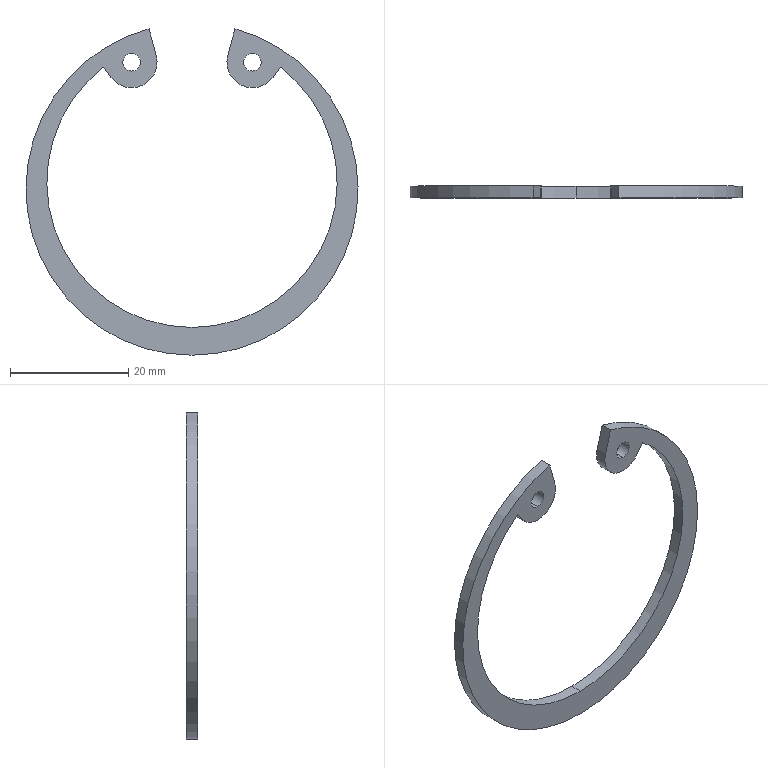Part | SolidWorks | features Extrusion 1 | 1 solid | 18 faces | box 56.2 x 2 x 55.243 mm | volume 1250 mm3 | cylinder 12 | plane 6 | commonest cylinder face diameters 3 x4 8.62 x4 49.15 x2 56.2 x2
STEP:
#1=CARTESIAN_POINT('',(10.219,2.,19.984));
#2=VERTEX_POINT('',#1);
#3=CARTESIAN_POINT('',(10.219,2.,22.984));
#4=VERTEX_POINT('',#3);
#5=CARTESIAN_POINT('',(10.219,2.,21.484));
#6=DIRECTION('',(0.,1.,0.));
#7=DIRECTION('',(0.,0.,-1.));
#8=AXIS2_PLACEMENT_3D('',#5,#6,#7);
#9=CIRCLE('',#8,1.5);
#10=EDGE_CURVE('',#2,#4,#9,.T.);
#11=ORIENTED_EDGE('',*,*,#10,.T.);
#12=CARTESIAN_POINT('',(10.219,0.,22.984));
#13=VERTEX_POINT('',#12);
#14=CARTESIAN_POINT('',(10.219,2.,22.984));
#15=DIRECTION('',(0.,-1.,0.));
#16=VECTOR('',#15,1000.);
#17=LINE('',#14,#16);
#18=EDGE_CURVE('',#4,#13,#17,.T.);
#19=ORIENTED_EDGE('',*,*,#18,.T.);
#20=CARTESIAN_POINT('',(10.219,0.,19.984));
#21=VERTEX_POINT('',#20);
#22=CARTESIAN_POINT('',(10.219,0.,21.484));
#23=DIRECTION('',(0.,1.,0.));
#24=DIRECTION('',(0.,0.,-1.));
#25=AXIS2_PLACEMENT_3D('',#22,#23,#24);
#26=CIRCLE('',#25,1.5);
#27=EDGE_CURVE('',#21,#13,#26,.T.);
#28=ORIENTED_EDGE('',*,*,#27,.F.);
#29=CARTESIAN_POINT('',(10.219,2.,19.984));
#30=DIRECTION('',(0.,-1.,0.));
#31=VECTOR('',#30,1000.);
#32=LINE('',#29,#31);
#33=EDGE_CURVE('',#2,#21,#32,.T.);
#34=ORIENTED_EDGE('',*,*,#33,.F.);
#35=EDGE_LOOP('',(#11,#19,#28,#34));
#36=FACE_OUTER_BOUND('',#35,.T.);
#37=CARTESIAN_POINT('',(10.219,2.,21.484));
#38=DIRECTION('',(0.,-1.,0.));
#39=DIRECTION('',(0.,0.,-1.));
#40=AXIS2_PLACEMENT_3D('',#37,#38,#39);
#41=CYLINDRICAL_SURFACE('',#40,1.5);
#42=ADVANCED_FACE('',(#36),#41,.F.);
#43=CARTESIAN_POINT('',(-10.219,2.,19.984));
#44=VERTEX_POINT('',#43);
#45=CARTESIAN_POINT('',(-10.219,2.,22.984));
#46=VERTEX_POINT('',#45);
#47=CARTESIAN_POINT('',(-10.219,2.,21.484));
#48=DIRECTION('',(0.,1.,0.));
#49=DIRECTION('',(0.,0.,1.));
#50=AXIS2_PLACEMENT_3D('',#47,#48,#49);
#51=CIRCLE('',#50,1.5);
#52=EDGE_CURVE('',#44,#46,#51,.T.);
#53=ORIENTED_EDGE('',*,*,#52,.T.);
#54=CARTESIAN_POINT('',(-10.219,0.,22.984));
#55=VERTEX_POINT('',#54);
#56=CARTESIAN_POINT('',(-10.219,2.,22.984));
#57=DIRECTION('',(0.,-1.,0.));
#58=VECTOR('',#57,1000.);
#59=LINE('',#56,#58);
#60=EDGE_CURVE('',#46,#55,#59,.T.);
#61=ORIENTED_EDGE('',*,*,#60,.T.);
#62=CARTESIAN_POINT('',(-10.219,0.,19.984));
#63=VERTEX_POINT('',#62);
#64=CARTESIAN_POINT('',(-10.219,0.,21.484));
#65=DIRECTION('',(0.,1.,0.));
#66=DIRECTION('',(0.,0.,1.));
#67=AXIS2_PLACEMENT_3D('',#64,#65,#66);
#68=CIRCLE('',#67,1.5);
#69=EDGE_CURVE('',#63,#55,#68,.T.);
#70=ORIENTED_EDGE('',*,*,#69,.F.);
#71=CARTESIAN_POINT('',(-10.219,2.,19.984));
#72=DIRECTION('',(0.,-1.,0.));
#73=VECTOR('',#72,1000.);
#74=LINE('',#71,#73);
#75=EDGE_CURVE('',#44,#63,#74,.T.);
#76=ORIENTED_EDGE('',*,*,#75,.F.);
#77=EDGE_LOOP('',(#53,#61,#70,#76));
#78=FACE_OUTER_BOUND('',#77,.T.);
#79=CARTESIAN_POINT('',(-10.219,2.,21.484));
#80=DIRECTION('',(0.,-1.,0.));
#81=DIRECTION('',(0.,0.,-1.));
#82=AXIS2_PLACEMENT_3D('',#79,#80,#81);
#83=CYLINDRICAL_SURFACE('',#82,1.5);
#84=ADVANCED_FACE('',(#78),#83,.F.);
#85=CARTESIAN_POINT('',(0.,2.,-28.1));
#86=VERTEX_POINT('',#85);
#87=CARTESIAN_POINT('',(-7.273,2.,27.143));
#88=VERTEX_POINT('',#87);
#89=CARTESIAN_POINT('',(0.,2.,0.));
#90=DIRECTION('',(0.,1.,0.));
#91=DIRECTION('',(0.,0.,1.));
#92=AXIS2_PLACEMENT_3D('',#89,#90,#91);
#93=CIRCLE('',#92,28.1);
#94=EDGE_CURVE('',#86,#88,#93,.T.);
#95=ORIENTED_EDGE('',*,*,#94,.F.);
#96=CARTESIAN_POINT('',(0.,0.,-28.1));
#97=VERTEX_POINT('',#96);
#98=CARTESIAN_POINT('',(0.,2.,-28.1));
#99=DIRECTION('',(0.,-1.,0.));
#100=VECTOR('',#99,1000.);
#101=LINE('',#98,#100);
#102=EDGE_CURVE('',#86,#97,#101,.T.);
#103=ORIENTED_EDGE('',*,*,#102,.T.);
#104=CARTESIAN_POINT('',(-7.273,0.,27.143));
#105=VERTEX_POINT('',#104);
#106=CARTESIAN_POINT('',(0.,0.,0.));
#107=DIRECTION('',(0.,1.,0.));
#108=DIRECTION('',(0.,0.,1.));
#109=AXIS2_PLACEMENT_3D('',#106,#107,#108);
#110=CIRCLE('',#109,28.1);
#111=EDGE_CURVE('',#97,#105,#110,.T.);
#112=ORIENTED_EDGE('',*,*,#111,.T.);
#113=CARTESIAN_POINT('',(-7.273,2.,27.143));
#114=DIRECTION('',(0.,-1.,0.));
#115=VECTOR('',#114,1000.);
#116=LINE('',#113,#115);
#117=EDGE_CURVE('',#88,#105,#116,.T.);
#118=ORIENTED_EDGE('',*,*,#117,.F.);
#119=EDGE_LOOP('',(#95,#103,#112,#118));
#120=FACE_OUTER_BOUND('',#119,.T.);
#121=CARTESIAN_POINT('',(0.,2.,0.));
#122=DIRECTION('',(0.,-1.,0.));
#123=DIRECTION('',(0.,0.,-1.));
#124=AXIS2_PLACEMENT_3D('',#121,#122,#123);
#125=CYLINDRICAL_SURFACE('',#124,28.1);
#126=ADVANCED_FACE('',(#120),#125,.T.);
#127=CARTESIAN_POINT('',(10.219,2.,17.174));
#128=VERTEX_POINT('',#127);
#129=CARTESIAN_POINT('',(6.055,2.,22.599));
#130=VERTEX_POINT('',#129);
#131=CARTESIAN_POINT('',(10.219,2.,21.484));
#132=DIRECTION('',(0.,1.,0.));
#133=DIRECTION('',(0.,0.,-1.));
#134=AXIS2_PLACEMENT_3D('',#131,#132,#133);
#135=CIRCLE('',#134,4.31);
#136=EDGE_CURVE('',#128,#130,#135,.T.);
#137=ORIENTED_EDGE('',*,*,#136,.F.);
#138=CARTESIAN_POINT('',(10.219,0.,17.174));
#139=VERTEX_POINT('',#138);
#140=CARTESIAN_POINT('',(10.219,2.,17.174));
#141=DIRECTION('',(0.,-1.,0.));
#142=VECTOR('',#141,1000.);
#143=LINE('',#140,#142);
#144=EDGE_CURVE('',#128,#139,#143,.T.);
#145=ORIENTED_EDGE('',*,*,#144,.T.);
#146=CARTESIAN_POINT('',(6.055,0.,22.599));
#147=VERTEX_POINT('',#146);
#148=CARTESIAN_POINT('',(10.219,0.,21.484));
#149=DIRECTION('',(0.,1.,0.));
#150=DIRECTION('',(0.,0.,-1.));
#151=AXIS2_PLACEMENT_3D('',#148,#149,#150);
#152=CIRCLE('',#151,4.31);
#153=EDGE_CURVE('',#139,#147,#152,.T.);
#154=ORIENTED_EDGE('',*,*,#153,.T.);
#155=CARTESIAN_POINT('',(6.055,2.,22.599));
#156=DIRECTION('',(0.,-1.,0.));
#157=VECTOR('',#156,1000.);
#158=LINE('',#155,#157);
#159=EDGE_CURVE('',#130,#147,#158,.T.);
#160=ORIENTED_EDGE('',*,*,#159,.F.);
#161=EDGE_LOOP('',(#137,#145,#154,#160));
#162=FACE_OUTER_BOUND('',#161,.T.);
#163=CARTESIAN_POINT('',(10.219,2.,21.484));
#164=DIRECTION('',(0.,-1.,0.));
#165=DIRECTION('',(0.,0.,-1.));
#166=AXIS2_PLACEMENT_3D('',#163,#164,#165);
#167=CYLINDRICAL_SURFACE('',#166,4.31);
#168=ADVANCED_FACE('',(#162),#167,.T.);
#169=CARTESIAN_POINT('',(0.,2.,-23.4));
#170=VERTEX_POINT('',#169);
#171=CARTESIAN_POINT('',(14.954,2.,20.677));
#172=VERTEX_POINT('',#171);
#173=CARTESIAN_POINT('',(0.,2.,1.175));
#174=DIRECTION('',(0.,-1.,0.));
#175=DIRECTION('',(0.,0.,1.));
#176=AXIS2_PLACEMENT_3D('',#173,#174,#175);
#177=CIRCLE('',#176,24.575);
#178=EDGE_CURVE('',#170,#172,#177,.T.);
#179=ORIENTED_EDGE('',*,*,#178,.F.);
#180=CARTESIAN_POINT('',(0.,0.,-23.4));
#181=VERTEX_POINT('',#180);
#182=CARTESIAN_POINT('',(0.,2.,-23.4));
#183=DIRECTION('',(0.,-1.,0.));
#184=VECTOR('',#183,1000.);
#185=LINE('',#182,#184);
#186=EDGE_CURVE('',#170,#181,#185,.T.);
#187=ORIENTED_EDGE('',*,*,#186,.T.);
#188=CARTESIAN_POINT('',(14.954,0.,20.677));
#189=VERTEX_POINT('',#188);
#190=CARTESIAN_POINT('',(0.,0.,1.175));
#191=DIRECTION('',(0.,-1.,0.));
#192=DIRECTION('',(0.,0.,1.));
#193=AXIS2_PLACEMENT_3D('',#190,#191,#192);
#194=CIRCLE('',#193,24.575);
#195=EDGE_CURVE('',#181,#189,#194,.T.);
#196=ORIENTED_EDGE('',*,*,#195,.T.);
#197=CARTESIAN_POINT('',(14.954,2.,20.677));
#198=DIRECTION('',(0.,-1.,0.));
#199=VECTOR('',#198,1000.);
#200=LINE('',#197,#199);
#201=EDGE_CURVE('',#172,#189,#200,.T.);
#202=ORIENTED_EDGE('',*,*,#201,.F.);
#203=EDGE_LOOP('',(#179,#187,#196,#202));
#204=FACE_OUTER_BOUND('',#203,.T.);
#205=CARTESIAN_POINT('',(0.,2.,1.175));
#206=DIRECTION('',(0.,-1.,0.));
#207=DIRECTION('',(0.,0.,-1.));
#208=AXIS2_PLACEMENT_3D('',#205,#206,#207);
#209=CYLINDRICAL_SURFACE('',#208,24.575);
#210=ADVANCED_FACE('',(#204),#209,.F.);
#211=CARTESIAN_POINT('',(-10.219,2.,17.174));
#212=VERTEX_POINT('',#211);
#213=CARTESIAN_POINT('',(-13.711,2.,18.958));
#214=VERTEX_POINT('',#213);
#215=CARTESIAN_POINT('',(-10.219,2.,21.484));
#216=DIRECTION('',(0.,1.,0.));
#217=DIRECTION('',(0.,0.,1.));
#218=AXIS2_PLACEMENT_3D('',#215,#216,#217);
#219=CIRCLE('',#218,4.31);
#220=EDGE_CURVE('',#212,#214,#219,.T.);
#221=ORIENTED_EDGE('',*,*,#220,.F.);
#222=CARTESIAN_POINT('',(-10.219,0.,17.174));
#223=VERTEX_POINT('',#222);
#224=CARTESIAN_POINT('',(-10.219,2.,17.174));
#225=DIRECTION('',(0.,-1.,0.));
#226=VECTOR('',#225,1000.);
#227=LINE('',#224,#226);
#228=EDGE_CURVE('',#212,#223,#227,.T.);
#229=ORIENTED_EDGE('',*,*,#228,.T.);
#230=CARTESIAN_POINT('',(-13.711,0.,18.958));
#231=VERTEX_POINT('',#230);
#232=CARTESIAN_POINT('',(-10.219,0.,21.484));
#233=DIRECTION('',(0.,1.,0.));
#234=DIRECTION('',(0.,0.,1.));
#235=AXIS2_PLACEMENT_3D('',#232,#233,#234);
#236=CIRCLE('',#235,4.31);
#237=EDGE_CURVE('',#223,#231,#236,.T.);
#238=ORIENTED_EDGE('',*,*,#237,.T.);
#239=CARTESIAN_POINT('',(-13.711,2.,18.958));
#240=DIRECTION('',(0.,-1.,0.));
#241=VECTOR('',#240,1000.);
#242=LINE('',#239,#241);
#243=EDGE_CURVE('',#214,#231,#242,.T.);
#244=ORIENTED_EDGE('',*,*,#243,.F.);
#245=EDGE_LOOP('',(#221,#229,#238,#244));
#246=FACE_OUTER_BOUND('',#245,.T.);
#247=CARTESIAN_POINT('',(-10.219,2.,21.484));
#248=DIRECTION('',(0.,-1.,0.));
#249=DIRECTION('',(0.,0.,-1.));
#250=AXIS2_PLACEMENT_3D('',#247,#248,#249);
#251=CYLINDRICAL_SURFACE('',#250,4.31);
#252=ADVANCED_FACE('',(#246),#251,.T.);
#253=ORIENTED_EDGE('',*,*,#52,.F.);
#254=CARTESIAN_POINT('',(-10.219,2.,21.484));
#255=DIRECTION('',(0.,1.,0.));
#256=DIRECTION('',(0.,0.,1.));
#257=AXIS2_PLACEMENT_3D('',#254,#255,#256);
#258=CIRCLE('',#257,1.5);
#259=EDGE_CURVE('',#46,#44,#258,.T.);
#260=ORIENTED_EDGE('',*,*,#259,.F.);
#261=EDGE_LOOP('',(#253,#260));
#262=FACE_BOUND('',#261,.T.);
#263=CARTESIAN_POINT('',(-6.055,2.,22.599));
#264=VERTEX_POINT('',#263);
#265=CARTESIAN_POINT('',(-10.219,2.,21.484));
#266=DIRECTION('',(0.,1.,0.));
#267=DIRECTION('',(0.,0.,1.));
#268=AXIS2_PLACEMENT_3D('',#265,#266,#267);
#269=CIRCLE('',#268,4.31);
#270=EDGE_CURVE('',#264,#212,#269,.T.);
#271=ORIENTED_EDGE('',*,*,#270,.T.);
#272=ORIENTED_EDGE('',*,*,#220,.T.);
#273=CARTESIAN_POINT('',(-14.954,2.,20.677));
#274=VERTEX_POINT('',#273);
#275=CARTESIAN_POINT('',(-14.954,2.,20.677));
#276=DIRECTION('',(-0.586,0.,0.8103));
#277=VECTOR('',#276,1000.);
#278=LINE('',#275,#277);
#279=EDGE_CURVE('',#214,#274,#278,.T.);
#280=ORIENTED_EDGE('',*,*,#279,.T.);
#281=CARTESIAN_POINT('',(0.,2.,1.175));
#282=DIRECTION('',(0.,-1.,0.));
#283=DIRECTION('',(0.,0.,1.));
#284=AXIS2_PLACEMENT_3D('',#281,#282,#283);
#285=CIRCLE('',#284,24.575);
#286=EDGE_CURVE('',#274,#170,#285,.T.);
#287=ORIENTED_EDGE('',*,*,#286,.T.);
#288=ORIENTED_EDGE('',*,*,#178,.T.);
#289=CARTESIAN_POINT('',(13.711,2.,18.958));
#290=VERTEX_POINT('',#289);
#291=CARTESIAN_POINT('',(14.954,2.,20.677));
#292=DIRECTION('',(-0.586,0.,-0.8103));
#293=VECTOR('',#292,1000.);
#294=LINE('',#291,#293);
#295=EDGE_CURVE('',#172,#290,#294,.T.);
#296=ORIENTED_EDGE('',*,*,#295,.T.);
#297=CARTESIAN_POINT('',(10.219,2.,21.484));
#298=DIRECTION('',(0.,1.,0.));
#299=DIRECTION('',(0.,0.,-1.));
#300=AXIS2_PLACEMENT_3D('',#297,#298,#299);
#301=CIRCLE('',#300,4.31);
#302=EDGE_CURVE('',#290,#128,#301,.T.);
#303=ORIENTED_EDGE('',*,*,#302,.T.);
#304=ORIENTED_EDGE('',*,*,#136,.T.);
#305=CARTESIAN_POINT('',(7.273,2.,27.143));
#306=VERTEX_POINT('',#305);
#307=CARTESIAN_POINT('',(6.055,2.,22.599));
#308=DIRECTION('',(0.2588,0.,0.9659));
#309=VECTOR('',#308,1000.);
#310=LINE('',#307,#309);
#311=EDGE_CURVE('',#130,#306,#310,.T.);
#312=ORIENTED_EDGE('',*,*,#311,.T.);
#313=CARTESIAN_POINT('',(0.,2.,0.));
#314=DIRECTION('',(0.,1.,0.));
#315=DIRECTION('',(0.,0.,1.));
#316=AXIS2_PLACEMENT_3D('',#313,#314,#315);
#317=CIRCLE('',#316,28.1);
#318=EDGE_CURVE('',#306,#86,#317,.T.);
#319=ORIENTED_EDGE('',*,*,#318,.T.);
#320=ORIENTED_EDGE('',*,*,#94,.T.);
#321=CARTESIAN_POINT('',(-6.055,2.,22.599));
#322=DIRECTION('',(0.2588,0.,-0.9659));
#323=VECTOR('',#322,1000.);
#324=LINE('',#321,#323);
#325=EDGE_CURVE('',#88,#264,#324,.T.);
#326=ORIENTED_EDGE('',*,*,#325,.T.);
#327=EDGE_LOOP('',(#271,#272,#280,#287,#288,#296,#303,#304,#312,#319,#320,#326));
#328=FACE_OUTER_BOUND('',#327,.T.);
#329=ORIENTED_EDGE('',*,*,#10,.F.);
#330=CARTESIAN_POINT('',(10.219,2.,21.484));
#331=DIRECTION('',(0.,1.,0.));
#332=DIRECTION('',(0.,0.,-1.));
#333=AXIS2_PLACEMENT_3D('',#330,#331,#332);
#334=CIRCLE('',#333,1.5);
#335=EDGE_CURVE('',#4,#2,#334,.T.);
#336=ORIENTED_EDGE('',*,*,#335,.F.);
#337=EDGE_LOOP('',(#329,#336));
#338=FACE_BOUND('',#337,.T.);
#339=CARTESIAN_POINT('',(-10.219,2.,21.484));
#340=DIRECTION('',(0.,1.,0.));
#341=DIRECTION('',(0.,0.,1.));
#342=AXIS2_PLACEMENT_3D('',#339,#340,#341);
#343=PLANE('',#342);
#344=ADVANCED_FACE('',(#262,#328,#338),#343,.T.);
#345=CARTESIAN_POINT('',(-6.055,0.,22.599));
#346=VERTEX_POINT('',#345);
#347=CARTESIAN_POINT('',(-10.219,0.,21.484));
#348=DIRECTION('',(0.,1.,0.));
#349=DIRECTION('',(0.,0.,1.));
#350=AXIS2_PLACEMENT_3D('',#347,#348,#349);
#351=CIRCLE('',#350,4.31);
#352=EDGE_CURVE('',#346,#223,#351,.T.);
#353=ORIENTED_EDGE('',*,*,#352,.F.);
#354=CARTESIAN_POINT('',(-6.055,0.,22.599));
#355=DIRECTION('',(0.2588,0.,-0.9659));
#356=VECTOR('',#355,1000.);
#357=LINE('',#354,#356);
#358=EDGE_CURVE('',#105,#346,#357,.T.);
#359=ORIENTED_EDGE('',*,*,#358,.F.);
#360=ORIENTED_EDGE('',*,*,#111,.F.);
#361=CARTESIAN_POINT('',(7.273,0.,27.143));
#362=VERTEX_POINT('',#361);
#363=CARTESIAN_POINT('',(0.,0.,0.));
#364=DIRECTION('',(0.,1.,0.));
#365=DIRECTION('',(0.,0.,1.));
#366=AXIS2_PLACEMENT_3D('',#363,#364,#365);
#367=CIRCLE('',#366,28.1);
#368=EDGE_CURVE('',#362,#97,#367,.T.);
#369=ORIENTED_EDGE('',*,*,#368,.F.);
#370=CARTESIAN_POINT('',(6.055,0.,22.599));
#371=DIRECTION('',(0.2588,0.,0.9659));
#372=VECTOR('',#371,1000.);
#373=LINE('',#370,#372);
#374=EDGE_CURVE('',#147,#362,#373,.T.);
#375=ORIENTED_EDGE('',*,*,#374,.F.);
#376=ORIENTED_EDGE('',*,*,#153,.F.);
#377=CARTESIAN_POINT('',(13.711,0.,18.958));
#378=VERTEX_POINT('',#377);
#379=CARTESIAN_POINT('',(10.219,0.,21.484));
#380=DIRECTION('',(0.,1.,0.));
#381=DIRECTION('',(0.,0.,-1.));
#382=AXIS2_PLACEMENT_3D('',#379,#380,#381);
#383=CIRCLE('',#382,4.31);
#384=EDGE_CURVE('',#378,#139,#383,.T.);
#385=ORIENTED_EDGE('',*,*,#384,.F.);
#386=CARTESIAN_POINT('',(14.954,0.,20.677));
#387=DIRECTION('',(-0.586,0.,-0.8103));
#388=VECTOR('',#387,1000.);
#389=LINE('',#386,#388);
#390=EDGE_CURVE('',#189,#378,#389,.T.);
#391=ORIENTED_EDGE('',*,*,#390,.F.);
#392=ORIENTED_EDGE('',*,*,#195,.F.);
#393=CARTESIAN_POINT('',(-14.954,0.,20.677));
#394=VERTEX_POINT('',#393);
#395=CARTESIAN_POINT('',(0.,0.,1.175));
#396=DIRECTION('',(0.,-1.,0.));
#397=DIRECTION('',(0.,0.,1.));
#398=AXIS2_PLACEMENT_3D('',#395,#396,#397);
#399=CIRCLE('',#398,24.575);
#400=EDGE_CURVE('',#394,#181,#399,.T.);
#401=ORIENTED_EDGE('',*,*,#400,.F.);
#402=CARTESIAN_POINT('',(-14.954,0.,20.677));
#403=DIRECTION('',(-0.586,0.,0.8103));
#404=VECTOR('',#403,1000.);
#405=LINE('',#402,#404);
#406=EDGE_CURVE('',#231,#394,#405,.T.);
#407=ORIENTED_EDGE('',*,*,#406,.F.);
#408=ORIENTED_EDGE('',*,*,#237,.F.);
#409=EDGE_LOOP('',(#353,#359,#360,#369,#375,#376,#385,#391,#392,#401,#407,#408));
#410=FACE_OUTER_BOUND('',#409,.T.);
#411=ORIENTED_EDGE('',*,*,#69,.T.);
#412=CARTESIAN_POINT('',(-10.219,0.,21.484));
#413=DIRECTION('',(0.,1.,0.));
#414=DIRECTION('',(0.,0.,1.));
#415=AXIS2_PLACEMENT_3D('',#412,#413,#414);
#416=CIRCLE('',#415,1.5);
#417=EDGE_CURVE('',#55,#63,#416,.T.);
#418=ORIENTED_EDGE('',*,*,#417,.T.);
#419=EDGE_LOOP('',(#411,#418));
#420=FACE_BOUND('',#419,.T.);
#421=ORIENTED_EDGE('',*,*,#27,.T.);
#422=CARTESIAN_POINT('',(10.219,0.,21.484));
#423=DIRECTION('',(0.,1.,0.));
#424=DIRECTION('',(0.,0.,-1.));
#425=AXIS2_PLACEMENT_3D('',#422,#423,#424);
#426=CIRCLE('',#425,1.5);
#427=EDGE_CURVE('',#13,#21,#426,.T.);
#428=ORIENTED_EDGE('',*,*,#427,.T.);
#429=EDGE_LOOP('',(#421,#428));
#430=FACE_BOUND('',#429,.T.);
#431=CARTESIAN_POINT('',(-10.219,0.,21.484));
#432=DIRECTION('',(0.,1.,0.));
#433=DIRECTION('',(0.,0.,1.));
#434=AXIS2_PLACEMENT_3D('',#431,#432,#433);
#435=PLANE('',#434);
#436=ADVANCED_FACE('',(#410,#420,#430),#435,.F.);
#437=ORIENTED_EDGE('',*,*,#228,.F.);
#438=ORIENTED_EDGE('',*,*,#270,.F.);
#439=CARTESIAN_POINT('',(-6.055,2.,22.599));
#440=DIRECTION('',(0.,-1.,0.));
#441=VECTOR('',#440,1000.);
#442=LINE('',#439,#441);
#443=EDGE_CURVE('',#264,#346,#442,.T.);
#444=ORIENTED_EDGE('',*,*,#443,.T.);
#445=ORIENTED_EDGE('',*,*,#352,.T.);
#446=EDGE_LOOP('',(#437,#438,#444,#445));
#447=FACE_OUTER_BOUND('',#446,.T.);
#448=CARTESIAN_POINT('',(-10.219,2.,21.484));
#449=DIRECTION('',(0.,-1.,0.));
#450=DIRECTION('',(0.,0.,-1.));
#451=AXIS2_PLACEMENT_3D('',#448,#449,#450);
#452=CYLINDRICAL_SURFACE('',#451,4.31);
#453=ADVANCED_FACE('',(#447),#452,.T.);
#454=ORIENTED_EDGE('',*,*,#406,.T.);
#455=CARTESIAN_POINT('',(-14.954,2.,20.677));
#456=DIRECTION('',(0.,-1.,0.));
#457=VECTOR('',#456,1000.);
#458=LINE('',#455,#457);
#459=EDGE_CURVE('',#274,#394,#458,.T.);
#460=ORIENTED_EDGE('',*,*,#459,.F.);
#461=ORIENTED_EDGE('',*,*,#279,.F.);
#462=ORIENTED_EDGE('',*,*,#243,.T.);
#463=EDGE_LOOP('',(#454,#460,#461,#462));
#464=FACE_OUTER_BOUND('',#463,.T.);
#465=CARTESIAN_POINT('',(-14.954,2.,20.677));
#466=DIRECTION('',(0.8103,0.,0.586));
#467=DIRECTION('',(0.586,0.,-0.8103));
#468=AXIS2_PLACEMENT_3D('',#465,#466,#467);
#469=PLANE('',#468);
#470=ADVANCED_FACE('',(#464),#469,.F.);
#471=ORIENTED_EDGE('',*,*,#186,.F.);
#472=ORIENTED_EDGE('',*,*,#286,.F.);
#473=ORIENTED_EDGE('',*,*,#459,.T.);
#474=ORIENTED_EDGE('',*,*,#400,.T.);
#475=EDGE_LOOP('',(#471,#472,#473,#474));
#476=FACE_OUTER_BOUND('',#475,.T.);
#477=CARTESIAN_POINT('',(0.,2.,1.175));
#478=DIRECTION('',(0.,-1.,0.));
#479=DIRECTION('',(0.,0.,-1.));
#480=AXIS2_PLACEMENT_3D('',#477,#478,#479);
#481=CYLINDRICAL_SURFACE('',#480,24.575);
#482=ADVANCED_FACE('',(#476),#481,.F.);
#483=ORIENTED_EDGE('',*,*,#390,.T.);
#484=CARTESIAN_POINT('',(13.711,2.,18.958));
#485=DIRECTION('',(0.,-1.,0.));
#486=VECTOR('',#485,1000.);
#487=LINE('',#484,#486);
#488=EDGE_CURVE('',#290,#378,#487,.T.);
#489=ORIENTED_EDGE('',*,*,#488,.F.);
#490=ORIENTED_EDGE('',*,*,#295,.F.);
#491=ORIENTED_EDGE('',*,*,#201,.T.);
#492=EDGE_LOOP('',(#483,#489,#490,#491));
#493=FACE_OUTER_BOUND('',#492,.T.);
#494=CARTESIAN_POINT('',(14.954,2.,20.677));
#495=DIRECTION('',(-0.8103,0.,0.586));
#496=DIRECTION('',(0.586,0.,0.8103));
#497=AXIS2_PLACEMENT_3D('',#494,#495,#496);
#498=PLANE('',#497);
#499=ADVANCED_FACE('',(#493),#498,.F.);
#500=ORIENTED_EDGE('',*,*,#144,.F.);
#501=ORIENTED_EDGE('',*,*,#302,.F.);
#502=ORIENTED_EDGE('',*,*,#488,.T.);
#503=ORIENTED_EDGE('',*,*,#384,.T.);
#504=EDGE_LOOP('',(#500,#501,#502,#503));
#505=FACE_OUTER_BOUND('',#504,.T.);
#506=CARTESIAN_POINT('',(10.219,2.,21.484));
#507=DIRECTION('',(0.,-1.,0.));
#508=DIRECTION('',(0.,0.,-1.));
#509=AXIS2_PLACEMENT_3D('',#506,#507,#508);
#510=CYLINDRICAL_SURFACE('',#509,4.31);
#511=ADVANCED_FACE('',(#505),#510,.T.);
#512=ORIENTED_EDGE('',*,*,#374,.T.);
#513=CARTESIAN_POINT('',(7.273,2.,27.143));
#514=DIRECTION('',(0.,-1.,0.));
#515=VECTOR('',#514,1000.);
#516=LINE('',#513,#515);
#517=EDGE_CURVE('',#306,#362,#516,.T.);
#518=ORIENTED_EDGE('',*,*,#517,.F.);
#519=ORIENTED_EDGE('',*,*,#311,.F.);
#520=ORIENTED_EDGE('',*,*,#159,.T.);
#521=EDGE_LOOP('',(#512,#518,#519,#520));
#522=FACE_OUTER_BOUND('',#521,.T.);
#523=CARTESIAN_POINT('',(6.055,2.,22.599));
#524=DIRECTION('',(0.9659,0.,-0.2588));
#525=DIRECTION('',(-0.2588,0.,-0.9659));
#526=AXIS2_PLACEMENT_3D('',#523,#524,#525);
#527=PLANE('',#526);
#528=ADVANCED_FACE('',(#522),#527,.F.);
#529=ORIENTED_EDGE('',*,*,#102,.F.);
#530=ORIENTED_EDGE('',*,*,#318,.F.);
#531=ORIENTED_EDGE('',*,*,#517,.T.);
#532=ORIENTED_EDGE('',*,*,#368,.T.);
#533=EDGE_LOOP('',(#529,#530,#531,#532));
#534=FACE_OUTER_BOUND('',#533,.T.);
#535=CARTESIAN_POINT('',(0.,2.,0.));
#536=DIRECTION('',(0.,-1.,0.));
#537=DIRECTION('',(0.,0.,-1.));
#538=AXIS2_PLACEMENT_3D('',#535,#536,#537);
#539=CYLINDRICAL_SURFACE('',#538,28.1);
#540=ADVANCED_FACE('',(#534),#539,.T.);
#541=ORIENTED_EDGE('',*,*,#358,.T.);
#542=ORIENTED_EDGE('',*,*,#443,.F.);
#543=ORIENTED_EDGE('',*,*,#325,.F.);
#544=ORIENTED_EDGE('',*,*,#117,.T.);
#545=EDGE_LOOP('',(#541,#542,#543,#544));
#546=FACE_OUTER_BOUND('',#545,.T.);
#547=CARTESIAN_POINT('',(-6.055,2.,22.599));
#548=DIRECTION('',(-0.9659,0.,-0.2588));
#549=DIRECTION('',(-0.2588,0.,0.9659));
#550=AXIS2_PLACEMENT_3D('',#547,#548,#549);
#551=PLANE('',#550);
#552=ADVANCED_FACE('',(#546),#551,.F.);
#553=ORIENTED_EDGE('',*,*,#60,.F.);
#554=ORIENTED_EDGE('',*,*,#259,.T.);
#555=ORIENTED_EDGE('',*,*,#75,.T.);
#556=ORIENTED_EDGE('',*,*,#417,.F.);
#557=EDGE_LOOP('',(#553,#554,#555,#556));
#558=FACE_OUTER_BOUND('',#557,.T.);
#559=CARTESIAN_POINT('',(-10.219,2.,21.484));
#560=DIRECTION('',(0.,-1.,0.));
#561=DIRECTION('',(0.,0.,-1.));
#562=AXIS2_PLACEMENT_3D('',#559,#560,#561);
#563=CYLINDRICAL_SURFACE('',#562,1.5);
#564=ADVANCED_FACE('',(#558),#563,.F.);
#565=ORIENTED_EDGE('',*,*,#18,.F.);
#566=ORIENTED_EDGE('',*,*,#335,.T.);
#567=ORIENTED_EDGE('',*,*,#33,.T.);
#568=ORIENTED_EDGE('',*,*,#427,.F.);
#569=EDGE_LOOP('',(#565,#566,#567,#568));
#570=FACE_OUTER_BOUND('',#569,.T.);
#571=CARTESIAN_POINT('',(10.219,2.,21.484));
#572=DIRECTION('',(0.,-1.,0.));
#573=DIRECTION('',(0.,0.,-1.));
#574=AXIS2_PLACEMENT_3D('',#571,#572,#573);
#575=CYLINDRICAL_SURFACE('',#574,1.5);
#576=ADVANCED_FACE('',(#570),#575,.F.);
#577=CLOSED_SHELL('',(#42,#84,#126,#168,#210,#252,#344,#436,#453,#470,#482,#499,#511,#528,#540,#552,#564,#576));
#578=MANIFOLD_SOLID_BREP('',#577);
#579=CARTESIAN_POINT('',(0.,0.,0.));
#580=DIRECTION('',(0.,0.,1.));
#581=DIRECTION('',(1.,0.,0.));
#582=AXIS2_PLACEMENT_3D('',#579,#580,#581);
#583=(LENGTH_UNIT()NAMED_UNIT(*)SI_UNIT(.MILLI.,.METRE.));
#584=UNCERTAINTY_MEASURE_WITH_UNIT(LENGTH_MEASURE(0.00001),#583,'','');
#585=(NAMED_UNIT(*)PLANE_ANGLE_UNIT()SI_UNIT($,.RADIAN.));
#586=(NAMED_UNIT(*)SI_UNIT($,.STERADIAN.)SOLID_ANGLE_UNIT());
#587=(GEOMETRIC_REPRESENTATION_CONTEXT(3)GLOBAL_UNCERTAINTY_ASSIGNED_CONTEXT((#584))GLOBAL_UNIT_ASSIGNED_CONTEXT((#583,#585,#586))REPRESENTATION_CONTEXT('',''));
#588=ADVANCED_BREP_SHAPE_REPRESENTATION('',(#578,#582),#587);